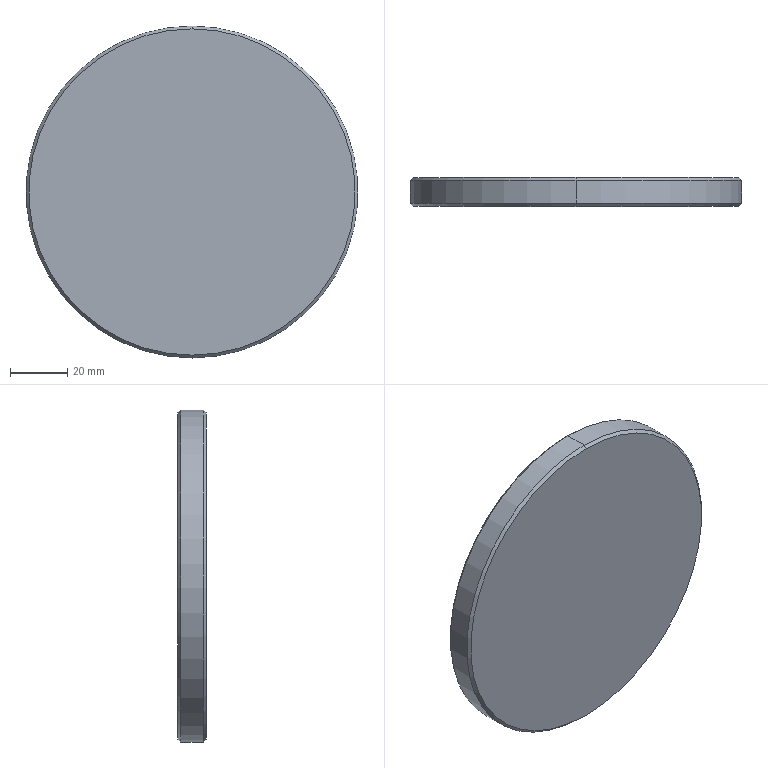Part | SolidWorks | features Chamfer 1, Extrusion 1 | 1 solid | 8 faces | box 116 x 10 x 116 mm | volume 105321 mm3 | cone 4 | cylinder 2 | plane 2 | commonest cylinder face diameters 116 x2
STEP:
#1=CARTESIAN_POINT('',(0.,10.,57.));
#2=VERTEX_POINT('',#1);
#3=CARTESIAN_POINT('',(0.,10.,-57.));
#4=VERTEX_POINT('',#3);
#5=CARTESIAN_POINT('',(0.,10.,0.));
#6=DIRECTION('',(0.,1.,0.));
#7=DIRECTION('',(0.,0.,1.));
#8=AXIS2_PLACEMENT_3D('',#5,#6,#7);
#9=CIRCLE('',#8,57.);
#10=EDGE_CURVE('',#2,#4,#9,.T.);
#11=ORIENTED_EDGE('',*,*,#10,.F.);
#12=CARTESIAN_POINT('',(0.,9.,58.));
#13=VERTEX_POINT('',#12);
#14=CARTESIAN_POINT('',(0.,10.,57.));
#15=DIRECTION('',(0.,-0.7071,0.7071));
#16=VECTOR('',#15,1000.);
#17=LINE('',#14,#16);
#18=EDGE_CURVE('',#2,#13,#17,.T.);
#19=ORIENTED_EDGE('',*,*,#18,.T.);
#20=CARTESIAN_POINT('',(0.,9.,-58.));
#21=VERTEX_POINT('',#20);
#22=CARTESIAN_POINT('',(0.,9.,0.));
#23=DIRECTION('',(0.,-1.,0.));
#24=DIRECTION('',(0.,0.,1.));
#25=AXIS2_PLACEMENT_3D('',#22,#23,#24);
#26=CIRCLE('',#25,58.);
#27=EDGE_CURVE('',#21,#13,#26,.T.);
#28=ORIENTED_EDGE('',*,*,#27,.F.);
#29=CARTESIAN_POINT('',(0.,10.,-57.));
#30=DIRECTION('',(0.,-0.7071,-0.7071));
#31=VECTOR('',#30,1000.);
#32=LINE('',#29,#31);
#33=EDGE_CURVE('',#4,#21,#32,.T.);
#34=ORIENTED_EDGE('',*,*,#33,.F.);
#35=EDGE_LOOP('',(#11,#19,#28,#34));
#36=FACE_OUTER_BOUND('',#35,.T.);
#37=CARTESIAN_POINT('',(0.,10.,0.));
#38=DIRECTION('',(0.,-1.,0.));
#39=DIRECTION('',(0.,0.,-1.));
#40=AXIS2_PLACEMENT_3D('',#37,#38,#39);
#41=CONICAL_SURFACE('',#40,57.,0.7854);
#42=ADVANCED_FACE('',(#36),#41,.T.);
#43=CARTESIAN_POINT('',(0.,0.,-57.));
#44=VERTEX_POINT('',#43);
#45=CARTESIAN_POINT('',(0.,0.,57.));
#46=VERTEX_POINT('',#45);
#47=CARTESIAN_POINT('',(0.,0.,0.));
#48=DIRECTION('',(0.,-1.,0.));
#49=DIRECTION('',(0.,0.,1.));
#50=AXIS2_PLACEMENT_3D('',#47,#48,#49);
#51=CIRCLE('',#50,57.);
#52=EDGE_CURVE('',#44,#46,#51,.T.);
#53=ORIENTED_EDGE('',*,*,#52,.F.);
#54=CARTESIAN_POINT('',(0.,1.,-58.));
#55=VERTEX_POINT('',#54);
#56=CARTESIAN_POINT('',(0.,1.,-58.));
#57=DIRECTION('',(0.,0.7071,-0.7071));
#58=VECTOR('',#57,1000.);
#59=LINE('',#56,#58);
#60=EDGE_CURVE('',#44,#55,#59,.T.);
#61=ORIENTED_EDGE('',*,*,#60,.T.);
#62=CARTESIAN_POINT('',(0.,1.,58.));
#63=VERTEX_POINT('',#62);
#64=CARTESIAN_POINT('',(0.,1.,0.));
#65=DIRECTION('',(0.,1.,0.));
#66=DIRECTION('',(0.,0.,1.));
#67=AXIS2_PLACEMENT_3D('',#64,#65,#66);
#68=CIRCLE('',#67,58.);
#69=EDGE_CURVE('',#63,#55,#68,.T.);
#70=ORIENTED_EDGE('',*,*,#69,.F.);
#71=CARTESIAN_POINT('',(0.,1.,58.));
#72=DIRECTION('',(0.,0.7071,0.7071));
#73=VECTOR('',#72,1000.);
#74=LINE('',#71,#73);
#75=EDGE_CURVE('',#46,#63,#74,.T.);
#76=ORIENTED_EDGE('',*,*,#75,.F.);
#77=EDGE_LOOP('',(#53,#61,#70,#76));
#78=FACE_OUTER_BOUND('',#77,.T.);
#79=CARTESIAN_POINT('',(0.,1.,0.));
#80=DIRECTION('',(0.,1.,0.));
#81=DIRECTION('',(0.,0.,1.));
#82=AXIS2_PLACEMENT_3D('',#79,#80,#81);
#83=CONICAL_SURFACE('',#82,58.,0.7854);
#84=ADVANCED_FACE('',(#78),#83,.T.);
#85=ORIENTED_EDGE('',*,*,#27,.T.);
#86=CARTESIAN_POINT('',(0.,10.,58.));
#87=DIRECTION('',(0.,-1.,0.));
#88=VECTOR('',#87,1000.);
#89=LINE('',#86,#88);
#90=EDGE_CURVE('',#13,#63,#89,.T.);
#91=ORIENTED_EDGE('',*,*,#90,.T.);
#92=ORIENTED_EDGE('',*,*,#69,.T.);
#93=CARTESIAN_POINT('',(0.,10.,-58.));
#94=DIRECTION('',(0.,-1.,0.));
#95=VECTOR('',#94,1000.);
#96=LINE('',#93,#95);
#97=EDGE_CURVE('',#21,#55,#96,.T.);
#98=ORIENTED_EDGE('',*,*,#97,.F.);
#99=EDGE_LOOP('',(#85,#91,#92,#98));
#100=FACE_OUTER_BOUND('',#99,.T.);
#101=CARTESIAN_POINT('',(0.,10.,0.));
#102=DIRECTION('',(0.,-1.,0.));
#103=DIRECTION('',(0.,0.,-1.));
#104=AXIS2_PLACEMENT_3D('',#101,#102,#103);
#105=CYLINDRICAL_SURFACE('',#104,58.);
#106=ADVANCED_FACE('',(#100),#105,.T.);
#107=ORIENTED_EDGE('',*,*,#90,.F.);
#108=CARTESIAN_POINT('',(0.,9.,0.));
#109=DIRECTION('',(0.,-1.,0.));
#110=DIRECTION('',(0.,0.,1.));
#111=AXIS2_PLACEMENT_3D('',#108,#109,#110);
#112=CIRCLE('',#111,58.);
#113=EDGE_CURVE('',#13,#21,#112,.T.);
#114=ORIENTED_EDGE('',*,*,#113,.T.);
#115=ORIENTED_EDGE('',*,*,#97,.T.);
#116=CARTESIAN_POINT('',(0.,1.,0.));
#117=DIRECTION('',(0.,1.,0.));
#118=DIRECTION('',(0.,0.,1.));
#119=AXIS2_PLACEMENT_3D('',#116,#117,#118);
#120=CIRCLE('',#119,58.);
#121=EDGE_CURVE('',#55,#63,#120,.T.);
#122=ORIENTED_EDGE('',*,*,#121,.T.);
#123=EDGE_LOOP('',(#107,#114,#115,#122));
#124=FACE_OUTER_BOUND('',#123,.T.);
#125=CARTESIAN_POINT('',(0.,10.,0.));
#126=DIRECTION('',(0.,-1.,0.));
#127=DIRECTION('',(0.,0.,-1.));
#128=AXIS2_PLACEMENT_3D('',#125,#126,#127);
#129=CYLINDRICAL_SURFACE('',#128,58.);
#130=ADVANCED_FACE('',(#124),#129,.T.);
#131=CARTESIAN_POINT('',(0.,10.,0.));
#132=DIRECTION('',(0.,1.,0.));
#133=DIRECTION('',(0.,0.,1.));
#134=AXIS2_PLACEMENT_3D('',#131,#132,#133);
#135=CIRCLE('',#134,57.);
#136=EDGE_CURVE('',#4,#2,#135,.T.);
#137=ORIENTED_EDGE('',*,*,#136,.T.);
#138=ORIENTED_EDGE('',*,*,#10,.T.);
#139=EDGE_LOOP('',(#137,#138));
#140=FACE_OUTER_BOUND('',#139,.T.);
#141=CARTESIAN_POINT('',(0.,10.,0.));
#142=DIRECTION('',(0.,1.,0.));
#143=DIRECTION('',(0.,0.,1.));
#144=AXIS2_PLACEMENT_3D('',#141,#142,#143);
#145=PLANE('',#144);
#146=ADVANCED_FACE('',(#140),#145,.T.);
#147=CARTESIAN_POINT('',(0.,0.,0.));
#148=DIRECTION('',(0.,-1.,0.));
#149=DIRECTION('',(0.,0.,1.));
#150=AXIS2_PLACEMENT_3D('',#147,#148,#149);
#151=CIRCLE('',#150,57.);
#152=EDGE_CURVE('',#46,#44,#151,.T.);
#153=ORIENTED_EDGE('',*,*,#152,.T.);
#154=ORIENTED_EDGE('',*,*,#52,.T.);
#155=EDGE_LOOP('',(#153,#154));
#156=FACE_OUTER_BOUND('',#155,.T.);
#157=CARTESIAN_POINT('',(0.,0.,0.));
#158=DIRECTION('',(0.,1.,0.));
#159=DIRECTION('',(0.,0.,1.));
#160=AXIS2_PLACEMENT_3D('',#157,#158,#159);
#161=PLANE('',#160);
#162=ADVANCED_FACE('',(#156),#161,.F.);
#163=ORIENTED_EDGE('',*,*,#60,.F.);
#164=ORIENTED_EDGE('',*,*,#152,.F.);
#165=ORIENTED_EDGE('',*,*,#75,.T.);
#166=ORIENTED_EDGE('',*,*,#121,.F.);
#167=EDGE_LOOP('',(#163,#164,#165,#166));
#168=FACE_OUTER_BOUND('',#167,.T.);
#169=CARTESIAN_POINT('',(0.,1.,0.));
#170=DIRECTION('',(0.,1.,0.));
#171=DIRECTION('',(0.,0.,1.));
#172=AXIS2_PLACEMENT_3D('',#169,#170,#171);
#173=CONICAL_SURFACE('',#172,58.,0.7854);
#174=ADVANCED_FACE('',(#168),#173,.T.);
#175=ORIENTED_EDGE('',*,*,#18,.F.);
#176=ORIENTED_EDGE('',*,*,#136,.F.);
#177=ORIENTED_EDGE('',*,*,#33,.T.);
#178=ORIENTED_EDGE('',*,*,#113,.F.);
#179=EDGE_LOOP('',(#175,#176,#177,#178));
#180=FACE_OUTER_BOUND('',#179,.T.);
#181=CARTESIAN_POINT('',(0.,10.,0.));
#182=DIRECTION('',(0.,-1.,0.));
#183=DIRECTION('',(0.,0.,-1.));
#184=AXIS2_PLACEMENT_3D('',#181,#182,#183);
#185=CONICAL_SURFACE('',#184,57.,0.7854);
#186=ADVANCED_FACE('',(#180),#185,.T.);
#187=CLOSED_SHELL('',(#42,#84,#106,#130,#146,#162,#174,#186));
#188=MANIFOLD_SOLID_BREP('',#187);
#189=CARTESIAN_POINT('',(0.,0.,0.));
#190=DIRECTION('',(0.,0.,1.));
#191=DIRECTION('',(1.,0.,0.));
#192=AXIS2_PLACEMENT_3D('',#189,#190,#191);
#193=(LENGTH_UNIT()NAMED_UNIT(*)SI_UNIT(.MILLI.,.METRE.));
#194=UNCERTAINTY_MEASURE_WITH_UNIT(LENGTH_MEASURE(0.00001),#193,'','');
#195=(NAMED_UNIT(*)PLANE_ANGLE_UNIT()SI_UNIT($,.RADIAN.));
#196=(NAMED_UNIT(*)SI_UNIT($,.STERADIAN.)SOLID_ANGLE_UNIT());
#197=(GEOMETRIC_REPRESENTATION_CONTEXT(3)GLOBAL_UNCERTAINTY_ASSIGNED_CONTEXT((#194))GLOBAL_UNIT_ASSIGNED_CONTEXT((#193,#195,#196))REPRESENTATION_CONTEXT('',''));
#198=ADVANCED_BREP_SHAPE_REPRESENTATION('',(#188,#192),#197);